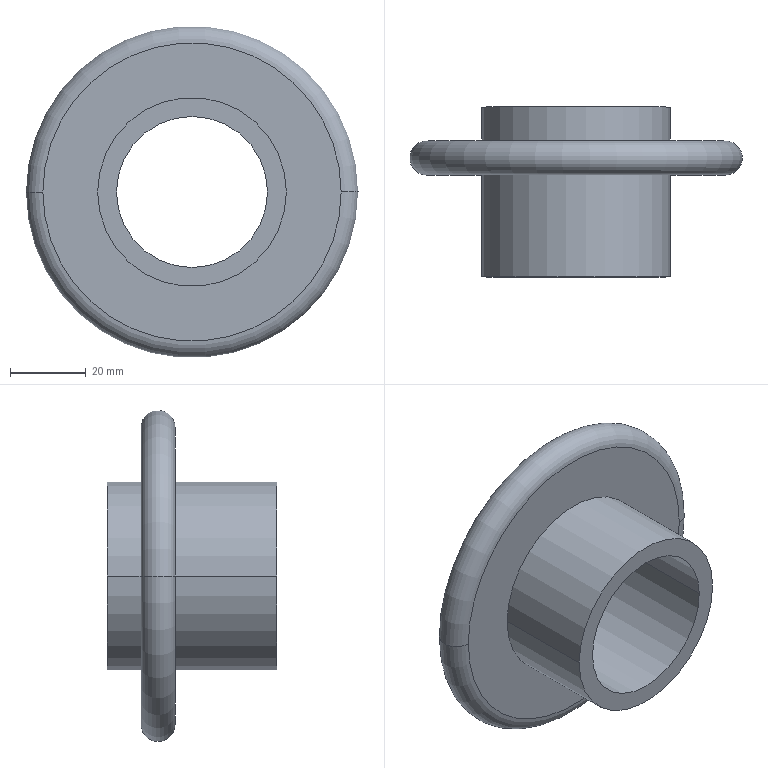Part | SolidWorks | features Revolution 1 | 1 solid | 12 faces | box 88 x 45 x 88 mm | volume 66528 mm3 | cylinder 6 | plane 4 | torus 2 | commonest cylinder face diameters 50 x4 40 x2
STEP:
#1=CARTESIAN_POINT('',(-25.,13.5,0.));
#2=VERTEX_POINT('',#1);
#3=CARTESIAN_POINT('',(25.,13.5,0.));
#4=VERTEX_POINT('',#3);
#5=CARTESIAN_POINT('',(0.,13.5,0.));
#6=DIRECTION('',(0.,1.,0.));
#7=DIRECTION('',(-1.,0.,0.));
#8=AXIS2_PLACEMENT_3D('',#5,#6,#7);
#9=CIRCLE('',#8,25.);
#10=EDGE_CURVE('',#2,#4,#9,.T.);
#11=ORIENTED_EDGE('',*,*,#10,.T.);
#12=CARTESIAN_POINT('',(25.,22.5,0.));
#13=VERTEX_POINT('',#12);
#14=CARTESIAN_POINT('',(25.,22.5,0.));
#15=DIRECTION('',(0.,1.,0.));
#16=VECTOR('',#15,1000.);
#17=LINE('',#14,#16);
#18=EDGE_CURVE('',#4,#13,#17,.T.);
#19=ORIENTED_EDGE('',*,*,#18,.T.);
#20=CARTESIAN_POINT('',(-25.,22.5,0.));
#21=VERTEX_POINT('',#20);
#22=CARTESIAN_POINT('',(0.,22.5,0.));
#23=DIRECTION('',(0.,1.,0.));
#24=DIRECTION('',(-1.,0.,0.));
#25=AXIS2_PLACEMENT_3D('',#22,#23,#24);
#26=CIRCLE('',#25,25.);
#27=EDGE_CURVE('',#21,#13,#26,.T.);
#28=ORIENTED_EDGE('',*,*,#27,.F.);
#29=CARTESIAN_POINT('',(-25.,22.5,0.));
#30=DIRECTION('',(0.,1.,0.));
#31=VECTOR('',#30,1000.);
#32=LINE('',#29,#31);
#33=EDGE_CURVE('',#2,#21,#32,.T.);
#34=ORIENTED_EDGE('',*,*,#33,.F.);
#35=EDGE_LOOP('',(#11,#19,#28,#34));
#36=FACE_OUTER_BOUND('',#35,.T.);
#37=CARTESIAN_POINT('',(0.,22.5,0.));
#38=DIRECTION('',(0.,1.,0.));
#39=DIRECTION('',(-1.,0.,0.));
#40=AXIS2_PLACEMENT_3D('',#37,#38,#39);
#41=CYLINDRICAL_SURFACE('',#40,25.);
#42=ADVANCED_FACE('',(#36),#41,.T.);
#43=CARTESIAN_POINT('',(-39.5,4.5,0.));
#44=VERTEX_POINT('',#43);
#45=CARTESIAN_POINT('',(39.5,4.5,0.));
#46=VERTEX_POINT('',#45);
#47=CARTESIAN_POINT('',(0.,4.5,0.));
#48=DIRECTION('',(0.,1.,0.));
#49=DIRECTION('',(-1.,0.,0.));
#50=AXIS2_PLACEMENT_3D('',#47,#48,#49);
#51=CIRCLE('',#50,39.5);
#52=EDGE_CURVE('',#44,#46,#51,.T.);
#53=ORIENTED_EDGE('',*,*,#52,.T.);
#54=CARTESIAN_POINT('',(39.5,13.5,0.));
#55=VERTEX_POINT('',#54);
#56=CARTESIAN_POINT('',(39.5,9.,0.));
#57=DIRECTION('',(0.,0.,1.));
#58=DIRECTION('',(1.,0.,0.));
#59=AXIS2_PLACEMENT_3D('',#56,#57,#58);
#60=CIRCLE('',#59,4.5);
#61=EDGE_CURVE('',#46,#55,#60,.T.);
#62=ORIENTED_EDGE('',*,*,#61,.T.);
#63=CARTESIAN_POINT('',(-39.5,13.5,0.));
#64=VERTEX_POINT('',#63);
#65=CARTESIAN_POINT('',(0.,13.5,0.));
#66=DIRECTION('',(0.,1.,0.));
#67=DIRECTION('',(-1.,0.,0.));
#68=AXIS2_PLACEMENT_3D('',#65,#66,#67);
#69=CIRCLE('',#68,39.5);
#70=EDGE_CURVE('',#64,#55,#69,.T.);
#71=ORIENTED_EDGE('',*,*,#70,.F.);
#72=CARTESIAN_POINT('',(-39.5,9.,0.));
#73=DIRECTION('',(0.,0.,-1.));
#74=DIRECTION('',(-1.,0.,0.));
#75=AXIS2_PLACEMENT_3D('',#72,#73,#74);
#76=CIRCLE('',#75,4.5);
#77=EDGE_CURVE('',#44,#64,#76,.T.);
#78=ORIENTED_EDGE('',*,*,#77,.F.);
#79=EDGE_LOOP('',(#53,#62,#71,#78));
#80=FACE_OUTER_BOUND('',#79,.T.);
#81=CARTESIAN_POINT('',(0.,9.,0.));
#82=DIRECTION('',(0.,1.,0.));
#83=DIRECTION('',(-1.,0.,0.));
#84=AXIS2_PLACEMENT_3D('',#81,#82,#83);
#85=TOROIDAL_SURFACE('',#84,39.5,4.5);
#86=ADVANCED_FACE('',(#80),#85,.T.);
#87=CARTESIAN_POINT('',(-25.,-22.5,0.));
#88=VERTEX_POINT('',#87);
#89=CARTESIAN_POINT('',(25.,-22.5,0.));
#90=VERTEX_POINT('',#89);
#91=CARTESIAN_POINT('',(0.,-22.5,0.));
#92=DIRECTION('',(0.,1.,0.));
#93=DIRECTION('',(-1.,0.,0.));
#94=AXIS2_PLACEMENT_3D('',#91,#92,#93);
#95=CIRCLE('',#94,25.);
#96=EDGE_CURVE('',#88,#90,#95,.T.);
#97=ORIENTED_EDGE('',*,*,#96,.T.);
#98=CARTESIAN_POINT('',(25.,4.5,0.));
#99=VERTEX_POINT('',#98);
#100=CARTESIAN_POINT('',(25.,22.5,0.));
#101=DIRECTION('',(0.,1.,0.));
#102=VECTOR('',#101,1000.);
#103=LINE('',#100,#102);
#104=EDGE_CURVE('',#90,#99,#103,.T.);
#105=ORIENTED_EDGE('',*,*,#104,.T.);
#106=CARTESIAN_POINT('',(-25.,4.5,0.));
#107=VERTEX_POINT('',#106);
#108=CARTESIAN_POINT('',(0.,4.5,0.));
#109=DIRECTION('',(0.,1.,0.));
#110=DIRECTION('',(-1.,0.,0.));
#111=AXIS2_PLACEMENT_3D('',#108,#109,#110);
#112=CIRCLE('',#111,25.);
#113=EDGE_CURVE('',#107,#99,#112,.T.);
#114=ORIENTED_EDGE('',*,*,#113,.F.);
#115=CARTESIAN_POINT('',(-25.,22.5,0.));
#116=DIRECTION('',(0.,1.,0.));
#117=VECTOR('',#116,1000.);
#118=LINE('',#115,#117);
#119=EDGE_CURVE('',#88,#107,#118,.T.);
#120=ORIENTED_EDGE('',*,*,#119,.F.);
#121=EDGE_LOOP('',(#97,#105,#114,#120));
#122=FACE_OUTER_BOUND('',#121,.T.);
#123=CARTESIAN_POINT('',(0.,22.5,0.));
#124=DIRECTION('',(0.,1.,0.));
#125=DIRECTION('',(-1.,0.,0.));
#126=AXIS2_PLACEMENT_3D('',#123,#124,#125);
#127=CYLINDRICAL_SURFACE('',#126,25.);
#128=ADVANCED_FACE('',(#122),#127,.T.);
#129=CARTESIAN_POINT('',(20.,-22.5,0.));
#130=VERTEX_POINT('',#129);
#131=CARTESIAN_POINT('',(-20.,-22.5,0.));
#132=VERTEX_POINT('',#131);
#133=CARTESIAN_POINT('',(0.,-22.5,0.));
#134=DIRECTION('',(0.,1.,0.));
#135=DIRECTION('',(-1.,0.,0.));
#136=AXIS2_PLACEMENT_3D('',#133,#134,#135);
#137=CIRCLE('',#136,20.);
#138=EDGE_CURVE('',#130,#132,#137,.T.);
#139=ORIENTED_EDGE('',*,*,#138,.F.);
#140=CARTESIAN_POINT('',(20.,22.5,0.));
#141=VERTEX_POINT('',#140);
#142=CARTESIAN_POINT('',(20.,22.5,0.));
#143=DIRECTION('',(0.,1.,0.));
#144=VECTOR('',#143,1000.);
#145=LINE('',#142,#144);
#146=EDGE_CURVE('',#130,#141,#145,.T.);
#147=ORIENTED_EDGE('',*,*,#146,.T.);
#148=CARTESIAN_POINT('',(-20.,22.5,0.));
#149=VERTEX_POINT('',#148);
#150=CARTESIAN_POINT('',(0.,22.5,0.));
#151=DIRECTION('',(0.,1.,0.));
#152=DIRECTION('',(-1.,0.,0.));
#153=AXIS2_PLACEMENT_3D('',#150,#151,#152);
#154=CIRCLE('',#153,20.);
#155=EDGE_CURVE('',#141,#149,#154,.T.);
#156=ORIENTED_EDGE('',*,*,#155,.T.);
#157=CARTESIAN_POINT('',(-20.,22.5,0.));
#158=DIRECTION('',(0.,1.,0.));
#159=VECTOR('',#158,1000.);
#160=LINE('',#157,#159);
#161=EDGE_CURVE('',#132,#149,#160,.T.);
#162=ORIENTED_EDGE('',*,*,#161,.F.);
#163=EDGE_LOOP('',(#139,#147,#156,#162));
#164=FACE_OUTER_BOUND('',#163,.T.);
#165=CARTESIAN_POINT('',(0.,22.5,0.));
#166=DIRECTION('',(0.,1.,0.));
#167=DIRECTION('',(-1.,0.,0.));
#168=AXIS2_PLACEMENT_3D('',#165,#166,#167);
#169=CYLINDRICAL_SURFACE('',#168,20.);
#170=ADVANCED_FACE('',(#164),#169,.F.);
#171=CARTESIAN_POINT('',(0.,22.5,0.));
#172=DIRECTION('',(0.,1.,0.));
#173=DIRECTION('',(-1.,0.,0.));
#174=AXIS2_PLACEMENT_3D('',#171,#172,#173);
#175=CIRCLE('',#174,20.);
#176=EDGE_CURVE('',#149,#141,#175,.T.);
#177=ORIENTED_EDGE('',*,*,#176,.F.);
#178=ORIENTED_EDGE('',*,*,#155,.F.);
#179=EDGE_LOOP('',(#177,#178));
#180=FACE_BOUND('',#179,.T.);
#181=ORIENTED_EDGE('',*,*,#27,.T.);
#182=CARTESIAN_POINT('',(0.,22.5,0.));
#183=DIRECTION('',(0.,1.,0.));
#184=DIRECTION('',(-1.,0.,0.));
#185=AXIS2_PLACEMENT_3D('',#182,#183,#184);
#186=CIRCLE('',#185,25.);
#187=EDGE_CURVE('',#13,#21,#186,.T.);
#188=ORIENTED_EDGE('',*,*,#187,.T.);
#189=EDGE_LOOP('',(#181,#188));
#190=FACE_OUTER_BOUND('',#189,.T.);
#191=CARTESIAN_POINT('',(25.,22.5,0.));
#192=DIRECTION('',(0.,-1.,0.));
#193=DIRECTION('',(1.,0.,0.));
#194=AXIS2_PLACEMENT_3D('',#191,#192,#193);
#195=PLANE('',#194);
#196=ADVANCED_FACE('',(#180,#190),#195,.F.);
#197=ORIENTED_EDGE('',*,*,#146,.F.);
#198=CARTESIAN_POINT('',(0.,-22.5,0.));
#199=DIRECTION('',(0.,1.,0.));
#200=DIRECTION('',(-1.,0.,0.));
#201=AXIS2_PLACEMENT_3D('',#198,#199,#200);
#202=CIRCLE('',#201,20.);
#203=EDGE_CURVE('',#132,#130,#202,.T.);
#204=ORIENTED_EDGE('',*,*,#203,.F.);
#205=ORIENTED_EDGE('',*,*,#161,.T.);
#206=ORIENTED_EDGE('',*,*,#176,.T.);
#207=EDGE_LOOP('',(#197,#204,#205,#206));
#208=FACE_OUTER_BOUND('',#207,.T.);
#209=CARTESIAN_POINT('',(0.,22.5,0.));
#210=DIRECTION('',(0.,1.,0.));
#211=DIRECTION('',(-1.,0.,0.));
#212=AXIS2_PLACEMENT_3D('',#209,#210,#211);
#213=CYLINDRICAL_SURFACE('',#212,20.);
#214=ADVANCED_FACE('',(#208),#213,.F.);
#215=ORIENTED_EDGE('',*,*,#96,.F.);
#216=CARTESIAN_POINT('',(0.,-22.5,0.));
#217=DIRECTION('',(0.,1.,0.));
#218=DIRECTION('',(-1.,0.,0.));
#219=AXIS2_PLACEMENT_3D('',#216,#217,#218);
#220=CIRCLE('',#219,25.);
#221=EDGE_CURVE('',#90,#88,#220,.T.);
#222=ORIENTED_EDGE('',*,*,#221,.F.);
#223=EDGE_LOOP('',(#215,#222));
#224=FACE_OUTER_BOUND('',#223,.T.);
#225=ORIENTED_EDGE('',*,*,#203,.T.);
#226=ORIENTED_EDGE('',*,*,#138,.T.);
#227=EDGE_LOOP('',(#225,#226));
#228=FACE_BOUND('',#227,.T.);
#229=CARTESIAN_POINT('',(20.,-22.5,0.));
#230=DIRECTION('',(0.,1.,0.));
#231=DIRECTION('',(-1.,0.,0.));
#232=AXIS2_PLACEMENT_3D('',#229,#230,#231);
#233=PLANE('',#232);
#234=ADVANCED_FACE('',(#224,#228),#233,.F.);
#235=ORIENTED_EDGE('',*,*,#104,.F.);
#236=ORIENTED_EDGE('',*,*,#221,.T.);
#237=ORIENTED_EDGE('',*,*,#119,.T.);
#238=CARTESIAN_POINT('',(0.,4.5,0.));
#239=DIRECTION('',(0.,1.,0.));
#240=DIRECTION('',(-1.,0.,0.));
#241=AXIS2_PLACEMENT_3D('',#238,#239,#240);
#242=CIRCLE('',#241,25.);
#243=EDGE_CURVE('',#99,#107,#242,.T.);
#244=ORIENTED_EDGE('',*,*,#243,.F.);
#245=EDGE_LOOP('',(#235,#236,#237,#244));
#246=FACE_OUTER_BOUND('',#245,.T.);
#247=CARTESIAN_POINT('',(0.,22.5,0.));
#248=DIRECTION('',(0.,1.,0.));
#249=DIRECTION('',(-1.,0.,0.));
#250=AXIS2_PLACEMENT_3D('',#247,#248,#249);
#251=CYLINDRICAL_SURFACE('',#250,25.);
#252=ADVANCED_FACE('',(#246),#251,.T.);
#253=ORIENTED_EDGE('',*,*,#52,.F.);
#254=CARTESIAN_POINT('',(0.,4.5,0.));
#255=DIRECTION('',(0.,1.,0.));
#256=DIRECTION('',(-1.,0.,0.));
#257=AXIS2_PLACEMENT_3D('',#254,#255,#256);
#258=CIRCLE('',#257,39.5);
#259=EDGE_CURVE('',#46,#44,#258,.T.);
#260=ORIENTED_EDGE('',*,*,#259,.F.);
#261=EDGE_LOOP('',(#253,#260));
#262=FACE_OUTER_BOUND('',#261,.T.);
#263=ORIENTED_EDGE('',*,*,#113,.T.);
#264=ORIENTED_EDGE('',*,*,#243,.T.);
#265=EDGE_LOOP('',(#263,#264));
#266=FACE_BOUND('',#265,.T.);
#267=CARTESIAN_POINT('',(25.,4.5,0.));
#268=DIRECTION('',(0.,1.,0.));
#269=DIRECTION('',(-1.,0.,0.));
#270=AXIS2_PLACEMENT_3D('',#267,#268,#269);
#271=PLANE('',#270);
#272=ADVANCED_FACE('',(#262,#266),#271,.F.);
#273=ORIENTED_EDGE('',*,*,#61,.F.);
#274=ORIENTED_EDGE('',*,*,#259,.T.);
#275=ORIENTED_EDGE('',*,*,#77,.T.);
#276=CARTESIAN_POINT('',(0.,13.5,0.));
#277=DIRECTION('',(0.,1.,0.));
#278=DIRECTION('',(-1.,0.,0.));
#279=AXIS2_PLACEMENT_3D('',#276,#277,#278);
#280=CIRCLE('',#279,39.5);
#281=EDGE_CURVE('',#55,#64,#280,.T.);
#282=ORIENTED_EDGE('',*,*,#281,.F.);
#283=EDGE_LOOP('',(#273,#274,#275,#282));
#284=FACE_OUTER_BOUND('',#283,.T.);
#285=CARTESIAN_POINT('',(0.,9.,0.));
#286=DIRECTION('',(0.,1.,0.));
#287=DIRECTION('',(-1.,0.,0.));
#288=AXIS2_PLACEMENT_3D('',#285,#286,#287);
#289=TOROIDAL_SURFACE('',#288,39.5,4.5);
#290=ADVANCED_FACE('',(#284),#289,.T.);
#291=ORIENTED_EDGE('',*,*,#10,.F.);
#292=CARTESIAN_POINT('',(0.,13.5,0.));
#293=DIRECTION('',(0.,1.,0.));
#294=DIRECTION('',(-1.,0.,0.));
#295=AXIS2_PLACEMENT_3D('',#292,#293,#294);
#296=CIRCLE('',#295,25.);
#297=EDGE_CURVE('',#4,#2,#296,.T.);
#298=ORIENTED_EDGE('',*,*,#297,.F.);
#299=EDGE_LOOP('',(#291,#298));
#300=FACE_BOUND('',#299,.T.);
#301=ORIENTED_EDGE('',*,*,#70,.T.);
#302=ORIENTED_EDGE('',*,*,#281,.T.);
#303=EDGE_LOOP('',(#301,#302));
#304=FACE_OUTER_BOUND('',#303,.T.);
#305=CARTESIAN_POINT('',(39.5,13.5,0.));
#306=DIRECTION('',(0.,-1.,0.));
#307=DIRECTION('',(1.,0.,0.));
#308=AXIS2_PLACEMENT_3D('',#305,#306,#307);
#309=PLANE('',#308);
#310=ADVANCED_FACE('',(#300,#304),#309,.F.);
#311=ORIENTED_EDGE('',*,*,#18,.F.);
#312=ORIENTED_EDGE('',*,*,#297,.T.);
#313=ORIENTED_EDGE('',*,*,#33,.T.);
#314=ORIENTED_EDGE('',*,*,#187,.F.);
#315=EDGE_LOOP('',(#311,#312,#313,#314));
#316=FACE_OUTER_BOUND('',#315,.T.);
#317=CARTESIAN_POINT('',(0.,22.5,0.));
#318=DIRECTION('',(0.,1.,0.));
#319=DIRECTION('',(-1.,0.,0.));
#320=AXIS2_PLACEMENT_3D('',#317,#318,#319);
#321=CYLINDRICAL_SURFACE('',#320,25.);
#322=ADVANCED_FACE('',(#316),#321,.T.);
#323=CLOSED_SHELL('',(#42,#86,#128,#170,#196,#214,#234,#252,#272,#290,#310,#322));
#324=MANIFOLD_SOLID_BREP('',#323);
#325=CARTESIAN_POINT('',(0.,0.,0.));
#326=DIRECTION('',(0.,0.,1.));
#327=DIRECTION('',(1.,0.,0.));
#328=AXIS2_PLACEMENT_3D('',#325,#326,#327);
#329=(LENGTH_UNIT()NAMED_UNIT(*)SI_UNIT(.MILLI.,.METRE.));
#330=UNCERTAINTY_MEASURE_WITH_UNIT(LENGTH_MEASURE(0.00001),#329,'','');
#331=(NAMED_UNIT(*)PLANE_ANGLE_UNIT()SI_UNIT($,.RADIAN.));
#332=(NAMED_UNIT(*)SI_UNIT($,.STERADIAN.)SOLID_ANGLE_UNIT());
#333=(GEOMETRIC_REPRESENTATION_CONTEXT(3)GLOBAL_UNCERTAINTY_ASSIGNED_CONTEXT((#330))GLOBAL_UNIT_ASSIGNED_CONTEXT((#329,#331,#332))REPRESENTATION_CONTEXT('',''));
#334=ADVANCED_BREP_SHAPE_REPRESENTATION('',(#324,#328),#333);